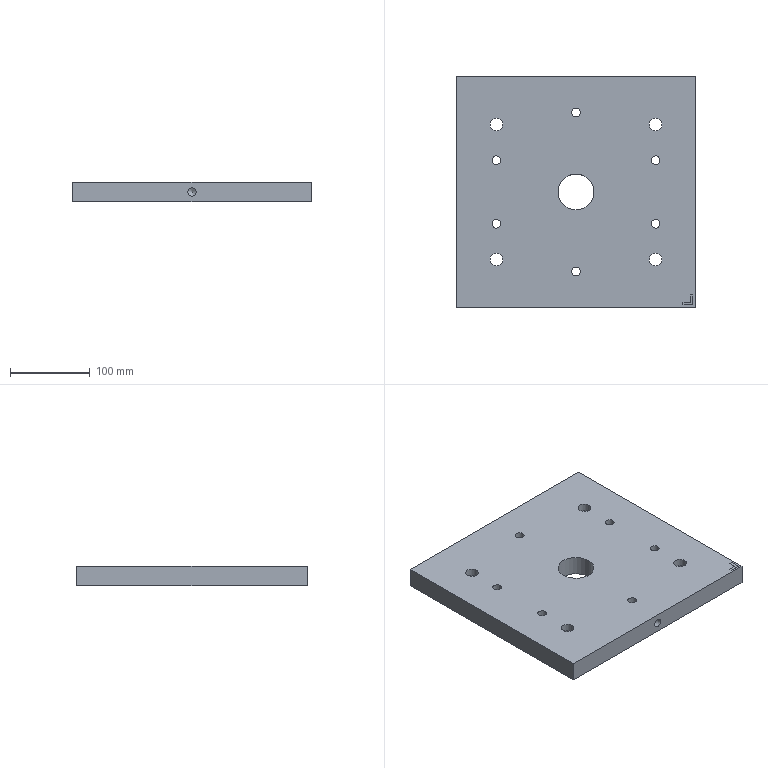Part | STEP file | BD_id262_x_t | 1 solid | 48 faces | box 300 x 290 x 25 mm | volume 2072800 mm3 | plane 23 | cylinder 23 | cone 2 | commonest cylinder face diameters 11 x6 18 x6 16 x4 23 x4 10.5 x2 45 x1
STEP:
#1=CARTESIAN_POINT('',(9.,100.,-190.5));
#2=VERTEX_POINT('',#1);
#3=CARTESIAN_POINT('',(0.,100.,-190.5));
#4=DIRECTION('',(0.,0.,1.));
#5=DIRECTION('',(1.,0.,0.));
#6=AXIS2_PLACEMENT_3D('',#3,#4,#5);
#7=CIRCLE('',#6,9.);
#8=EDGE_CURVE('',#2,#2,#7,.T.);
#9=ORIENTED_EDGE('',*,*,#8,.T.);
#10=EDGE_LOOP('',(#9));
#11=FACE_BOUND('',#10,.T.);
#12=CARTESIAN_POINT('',(-109.,-40.,-190.5));
#13=VERTEX_POINT('',#12);
#14=CARTESIAN_POINT('',(-100.,-40.,-190.5));
#15=DIRECTION('',(0.,0.,1.));
#16=DIRECTION('',(-1.,0.,0.));
#17=AXIS2_PLACEMENT_3D('',#14,#15,#16);
#18=CIRCLE('',#17,9.);
#19=EDGE_CURVE('',#13,#13,#18,.T.);
#20=ORIENTED_EDGE('',*,*,#19,.T.);
#21=EDGE_LOOP('',(#20));
#22=FACE_BOUND('',#21,.T.);
#23=CARTESIAN_POINT('',(109.,-40.,-190.5));
#24=VERTEX_POINT('',#23);
#25=CARTESIAN_POINT('',(100.,-40.,-190.5));
#26=DIRECTION('',(0.,0.,1.));
#27=DIRECTION('',(1.,0.,0.));
#28=AXIS2_PLACEMENT_3D('',#25,#26,#27);
#29=CIRCLE('',#28,9.);
#30=EDGE_CURVE('',#24,#24,#29,.T.);
#31=ORIENTED_EDGE('',*,*,#30,.T.);
#32=EDGE_LOOP('',(#31));
#33=FACE_BOUND('',#32,.T.);
#34=CARTESIAN_POINT('',(-111.5,-85.,-190.5));
#35=VERTEX_POINT('',#34);
#36=CARTESIAN_POINT('',(-100.,-85.,-190.5));
#37=DIRECTION('',(0.,0.,1.));
#38=DIRECTION('',(-1.,0.,0.));
#39=AXIS2_PLACEMENT_3D('',#36,#37,#38);
#40=CIRCLE('',#39,11.5);
#41=EDGE_CURVE('',#35,#35,#40,.T.);
#42=ORIENTED_EDGE('',*,*,#41,.T.);
#43=EDGE_LOOP('',(#42));
#44=FACE_BOUND('',#43,.T.);
#45=CARTESIAN_POINT('',(111.5,85.,-190.5));
#46=VERTEX_POINT('',#45);
#47=CARTESIAN_POINT('',(100.,85.,-190.5));
#48=DIRECTION('',(0.,0.,1.));
#49=DIRECTION('',(1.,0.,0.));
#50=AXIS2_PLACEMENT_3D('',#47,#48,#49);
#51=CIRCLE('',#50,11.5);
#52=EDGE_CURVE('',#46,#46,#51,.T.);
#53=ORIENTED_EDGE('',*,*,#52,.T.);
#54=EDGE_LOOP('',(#53));
#55=FACE_BOUND('',#54,.T.);
#56=CARTESIAN_POINT('',(150.,-145.,-190.5));
#57=VERTEX_POINT('',#56);
#58=CARTESIAN_POINT('',(150.,145.,-190.5));
#59=VERTEX_POINT('',#58);
#60=CARTESIAN_POINT('',(150.,0.,-190.5));
#61=DIRECTION('',(0.,1.,0.));
#62=VECTOR('',#61,1.);
#63=LINE('',#60,#62);
#64=EDGE_CURVE('',#57,#59,#63,.T.);
#65=ORIENTED_EDGE('',*,*,#64,.F.);
#66=CARTESIAN_POINT('',(-150.,-145.,-190.5));
#67=VERTEX_POINT('',#66);
#68=CARTESIAN_POINT('',(0.,-145.,-190.5));
#69=DIRECTION('',(1.,0.,0.));
#70=VECTOR('',#69,1.);
#71=LINE('',#68,#70);
#72=EDGE_CURVE('',#67,#57,#71,.T.);
#73=ORIENTED_EDGE('',*,*,#72,.F.);
#74=CARTESIAN_POINT('',(-150.,145.,-190.5));
#75=VERTEX_POINT('',#74);
#76=CARTESIAN_POINT('',(-150.,0.,-190.5));
#77=DIRECTION('',(0.,-1.,0.));
#78=VECTOR('',#77,1.);
#79=LINE('',#76,#78);
#80=EDGE_CURVE('',#75,#67,#79,.T.);
#81=ORIENTED_EDGE('',*,*,#80,.F.);
#82=CARTESIAN_POINT('',(0.,145.,-190.5));
#83=DIRECTION('',(-1.,0.,0.));
#84=VECTOR('',#83,1.);
#85=LINE('',#82,#84);
#86=EDGE_CURVE('',#59,#75,#85,.T.);
#87=ORIENTED_EDGE('',*,*,#86,.F.);
#88=EDGE_LOOP('',(#65,#73,#81,#87));
#89=FACE_BOUND('',#88,.T.);
#90=CARTESIAN_POINT('',(111.5,-85.,-190.5));
#91=VERTEX_POINT('',#90);
#92=CARTESIAN_POINT('',(100.,-85.,-190.5));
#93=DIRECTION('',(0.,0.,1.));
#94=DIRECTION('',(1.,0.,0.));
#95=AXIS2_PLACEMENT_3D('',#92,#93,#94);
#96=CIRCLE('',#95,11.5);
#97=EDGE_CURVE('',#91,#91,#96,.T.);
#98=ORIENTED_EDGE('',*,*,#97,.T.);
#99=EDGE_LOOP('',(#98));
#100=FACE_BOUND('',#99,.T.);
#101=CARTESIAN_POINT('',(-88.5,85.,-190.5));
#102=VERTEX_POINT('',#101);
#103=CARTESIAN_POINT('',(-100.,85.,-190.5));
#104=DIRECTION('',(0.,0.,1.));
#105=DIRECTION('',(1.,0.,0.));
#106=AXIS2_PLACEMENT_3D('',#103,#104,#105);
#107=CIRCLE('',#106,11.5);
#108=EDGE_CURVE('',#102,#102,#107,.T.);
#109=ORIENTED_EDGE('',*,*,#108,.T.);
#110=EDGE_LOOP('',(#109));
#111=FACE_BOUND('',#110,.T.);
#112=CARTESIAN_POINT('',(109.,40.,-190.5));
#113=VERTEX_POINT('',#112);
#114=CARTESIAN_POINT('',(100.,40.,-190.5));
#115=DIRECTION('',(0.,0.,1.));
#116=DIRECTION('',(1.,0.,0.));
#117=AXIS2_PLACEMENT_3D('',#114,#115,#116);
#118=CIRCLE('',#117,9.);
#119=EDGE_CURVE('',#113,#113,#118,.T.);
#120=ORIENTED_EDGE('',*,*,#119,.T.);
#121=EDGE_LOOP('',(#120));
#122=FACE_BOUND('',#121,.T.);
#123=CARTESIAN_POINT('',(-91.,40.,-190.5));
#124=VERTEX_POINT('',#123);
#125=CARTESIAN_POINT('',(-100.,40.,-190.5));
#126=DIRECTION('',(0.,0.,1.));
#127=DIRECTION('',(1.,0.,0.));
#128=AXIS2_PLACEMENT_3D('',#125,#126,#127);
#129=CIRCLE('',#128,9.);
#130=EDGE_CURVE('',#124,#124,#129,.T.);
#131=ORIENTED_EDGE('',*,*,#130,.T.);
#132=EDGE_LOOP('',(#131));
#133=FACE_BOUND('',#132,.T.);
#134=CARTESIAN_POINT('',(-22.5,0.,-190.5));
#135=VERTEX_POINT('',#134);
#136=CARTESIAN_POINT('',(0.,0.,-190.5));
#137=DIRECTION('',(0.,0.,1.));
#138=DIRECTION('',(-1.,0.,0.));
#139=AXIS2_PLACEMENT_3D('',#136,#137,#138);
#140=CIRCLE('',#139,22.5);
#141=EDGE_CURVE('',#135,#135,#140,.T.);
#142=ORIENTED_EDGE('',*,*,#141,.T.);
#143=EDGE_LOOP('',(#142));
#144=FACE_BOUND('',#143,.T.);
#145=CARTESIAN_POINT('',(9.,-100.,-190.5));
#146=VERTEX_POINT('',#145);
#147=CARTESIAN_POINT('',(0.,-100.,-190.5));
#148=DIRECTION('',(0.,0.,1.));
#149=DIRECTION('',(1.,0.,0.));
#150=AXIS2_PLACEMENT_3D('',#147,#148,#149);
#151=CIRCLE('',#150,9.);
#152=EDGE_CURVE('',#146,#146,#151,.T.);
#153=ORIENTED_EDGE('',*,*,#152,.T.);
#154=EDGE_LOOP('',(#153));
#155=FACE_BOUND('',#154,.T.);
#156=CARTESIAN_POINT('',(0.,0.,-190.5));
#157=DIRECTION('',(0.,0.,-1.));
#158=DIRECTION('',(-1.,0.,0.));
#159=AXIS2_PLACEMENT_3D('',#156,#157,#158);
#160=PLANE('',#159);
#161=ADVANCED_FACE('',(#11,#22,#33,#44,#55,#89,#100,#111,#122,#133,#144,#155),#160,.T.);
#162=CARTESIAN_POINT('',(-5.5,100.,-165.5));
#163=VERTEX_POINT('',#162);
#164=CARTESIAN_POINT('',(0.,100.,-165.5));
#165=DIRECTION('',(0.,0.,-1.));
#166=DIRECTION('',(-1.,0.,0.));
#167=AXIS2_PLACEMENT_3D('',#164,#165,#166);
#168=CIRCLE('',#167,5.5);
#169=EDGE_CURVE('',#163,#163,#168,.T.);
#170=ORIENTED_EDGE('',*,*,#169,.T.);
#171=EDGE_LOOP('',(#170));
#172=FACE_BOUND('',#171,.T.);
#173=CARTESIAN_POINT('',(-94.5,-40.,-165.5));
#174=VERTEX_POINT('',#173);
#175=CARTESIAN_POINT('',(-100.,-40.,-165.5));
#176=DIRECTION('',(0.,0.,-1.));
#177=DIRECTION('',(1.,0.,0.));
#178=AXIS2_PLACEMENT_3D('',#175,#176,#177);
#179=CIRCLE('',#178,5.5);
#180=EDGE_CURVE('',#174,#174,#179,.T.);
#181=ORIENTED_EDGE('',*,*,#180,.T.);
#182=EDGE_LOOP('',(#181));
#183=FACE_BOUND('',#182,.T.);
#184=CARTESIAN_POINT('',(94.5,-40.,-165.5));
#185=VERTEX_POINT('',#184);
#186=CARTESIAN_POINT('',(100.,-40.,-165.5));
#187=DIRECTION('',(0.,0.,-1.));
#188=DIRECTION('',(-1.,0.,0.));
#189=AXIS2_PLACEMENT_3D('',#186,#187,#188);
#190=CIRCLE('',#189,5.5);
#191=EDGE_CURVE('',#185,#185,#190,.T.);
#192=ORIENTED_EDGE('',*,*,#191,.T.);
#193=EDGE_LOOP('',(#192));
#194=FACE_BOUND('',#193,.T.);
#195=CARTESIAN_POINT('',(-92.,-85.,-165.5));
#196=VERTEX_POINT('',#195);
#197=CARTESIAN_POINT('',(-100.,-85.,-165.5));
#198=DIRECTION('',(0.,0.,-1.));
#199=DIRECTION('',(1.,0.,0.));
#200=AXIS2_PLACEMENT_3D('',#197,#198,#199);
#201=CIRCLE('',#200,8.);
#202=EDGE_CURVE('',#196,#196,#201,.T.);
#203=ORIENTED_EDGE('',*,*,#202,.T.);
#204=EDGE_LOOP('',(#203));
#205=FACE_BOUND('',#204,.T.);
#206=CARTESIAN_POINT('',(92.,85.,-165.5));
#207=VERTEX_POINT('',#206);
#208=CARTESIAN_POINT('',(100.,85.,-165.5));
#209=DIRECTION('',(0.,0.,-1.));
#210=DIRECTION('',(-1.,0.,0.));
#211=AXIS2_PLACEMENT_3D('',#208,#209,#210);
#212=CIRCLE('',#211,8.);
#213=EDGE_CURVE('',#207,#207,#212,.T.);
#214=ORIENTED_EDGE('',*,*,#213,.T.);
#215=EDGE_LOOP('',(#214));
#216=FACE_BOUND('',#215,.T.);
#217=CARTESIAN_POINT('',(143.75,-129.375,-165.5));
#218=VERTEX_POINT('',#217);
#219=CARTESIAN_POINT('',(143.75,-138.75,-165.5));
#220=VERTEX_POINT('',#219);
#221=CARTESIAN_POINT('',(143.75,-134.062,-165.5));
#222=DIRECTION('',(0.,-1.,0.));
#223=VECTOR('',#222,1.);
#224=LINE('',#221,#223);
#225=EDGE_CURVE('',#218,#220,#224,.T.);
#226=ORIENTED_EDGE('',*,*,#225,.F.);
#227=CARTESIAN_POINT('',(146.875,-129.375,-165.5));
#228=VERTEX_POINT('',#227);
#229=CARTESIAN_POINT('',(140.625,-129.375,-165.5));
#230=DIRECTION('',(1.,0.,0.));
#231=VECTOR('',#230,1.);
#232=LINE('',#229,#231);
#233=EDGE_CURVE('',#218,#228,#232,.T.);
#234=ORIENTED_EDGE('',*,*,#233,.T.);
#235=CARTESIAN_POINT('',(146.875,-141.875,-165.5));
#236=VERTEX_POINT('',#235);
#237=CARTESIAN_POINT('',(146.875,-135.625,-165.5));
#238=DIRECTION('',(0.,-1.,0.));
#239=VECTOR('',#238,1.);
#240=LINE('',#237,#239);
#241=EDGE_CURVE('',#228,#236,#240,.T.);
#242=ORIENTED_EDGE('',*,*,#241,.T.);
#243=CARTESIAN_POINT('',(134.375,-141.875,-165.5));
#244=VERTEX_POINT('',#243);
#245=CARTESIAN_POINT('',(140.625,-141.875,-165.5));
#246=DIRECTION('',(-1.,0.,0.));
#247=VECTOR('',#246,1.);
#248=LINE('',#245,#247);
#249=EDGE_CURVE('',#236,#244,#248,.T.);
#250=ORIENTED_EDGE('',*,*,#249,.T.);
#251=CARTESIAN_POINT('',(134.375,-138.75,-165.5));
#252=VERTEX_POINT('',#251);
#253=CARTESIAN_POINT('',(134.375,-135.625,-165.5));
#254=DIRECTION('',(0.,1.,0.));
#255=VECTOR('',#254,1.);
#256=LINE('',#253,#255);
#257=EDGE_CURVE('',#244,#252,#256,.T.);
#258=ORIENTED_EDGE('',*,*,#257,.T.);
#259=CARTESIAN_POINT('',(139.062,-138.75,-165.5));
#260=DIRECTION('',(-1.,0.,0.));
#261=VECTOR('',#260,1.);
#262=LINE('',#259,#261);
#263=EDGE_CURVE('',#220,#252,#262,.T.);
#264=ORIENTED_EDGE('',*,*,#263,.F.);
#265=EDGE_LOOP('',(#226,#234,#242,#250,#258,#264));
#266=FACE_BOUND('',#265,.T.);
#267=CARTESIAN_POINT('',(150.,-145.,-165.5));
#268=VERTEX_POINT('',#267);
#269=CARTESIAN_POINT('',(-150.,-145.,-165.5));
#270=VERTEX_POINT('',#269);
#271=CARTESIAN_POINT('',(0.,-145.,-165.5));
#272=DIRECTION('',(-1.,0.,0.));
#273=VECTOR('',#272,1.);
#274=LINE('',#271,#273);
#275=EDGE_CURVE('',#268,#270,#274,.T.);
#276=ORIENTED_EDGE('',*,*,#275,.F.);
#277=CARTESIAN_POINT('',(150.,145.,-165.5));
#278=VERTEX_POINT('',#277);
#279=CARTESIAN_POINT('',(150.,0.,-165.5));
#280=DIRECTION('',(0.,-1.,0.));
#281=VECTOR('',#280,1.);
#282=LINE('',#279,#281);
#283=EDGE_CURVE('',#278,#268,#282,.T.);
#284=ORIENTED_EDGE('',*,*,#283,.F.);
#285=CARTESIAN_POINT('',(-150.,145.,-165.5));
#286=VERTEX_POINT('',#285);
#287=CARTESIAN_POINT('',(0.,145.,-165.5));
#288=DIRECTION('',(1.,0.,0.));
#289=VECTOR('',#288,1.);
#290=LINE('',#287,#289);
#291=EDGE_CURVE('',#286,#278,#290,.T.);
#292=ORIENTED_EDGE('',*,*,#291,.F.);
#293=CARTESIAN_POINT('',(-150.,0.,-165.5));
#294=DIRECTION('',(0.,1.,0.));
#295=VECTOR('',#294,1.);
#296=LINE('',#293,#295);
#297=EDGE_CURVE('',#270,#286,#296,.T.);
#298=ORIENTED_EDGE('',*,*,#297,.F.);
#299=EDGE_LOOP('',(#276,#284,#292,#298));
#300=FACE_BOUND('',#299,.T.);
#301=CARTESIAN_POINT('',(92.,-85.,-165.5));
#302=VERTEX_POINT('',#301);
#303=CARTESIAN_POINT('',(100.,-85.,-165.5));
#304=DIRECTION('',(0.,0.,-1.));
#305=DIRECTION('',(-1.,0.,0.));
#306=AXIS2_PLACEMENT_3D('',#303,#304,#305);
#307=CIRCLE('',#306,8.);
#308=EDGE_CURVE('',#302,#302,#307,.T.);
#309=ORIENTED_EDGE('',*,*,#308,.T.);
#310=EDGE_LOOP('',(#309));
#311=FACE_BOUND('',#310,.T.);
#312=CARTESIAN_POINT('',(-108.,85.,-165.5));
#313=VERTEX_POINT('',#312);
#314=CARTESIAN_POINT('',(-100.,85.,-165.5));
#315=DIRECTION('',(0.,0.,-1.));
#316=DIRECTION('',(-1.,0.,0.));
#317=AXIS2_PLACEMENT_3D('',#314,#315,#316);
#318=CIRCLE('',#317,8.);
#319=EDGE_CURVE('',#313,#313,#318,.T.);
#320=ORIENTED_EDGE('',*,*,#319,.T.);
#321=EDGE_LOOP('',(#320));
#322=FACE_BOUND('',#321,.T.);
#323=CARTESIAN_POINT('',(94.5,40.,-165.5));
#324=VERTEX_POINT('',#323);
#325=CARTESIAN_POINT('',(100.,40.,-165.5));
#326=DIRECTION('',(0.,0.,-1.));
#327=DIRECTION('',(-1.,0.,0.));
#328=AXIS2_PLACEMENT_3D('',#325,#326,#327);
#329=CIRCLE('',#328,5.5);
#330=EDGE_CURVE('',#324,#324,#329,.T.);
#331=ORIENTED_EDGE('',*,*,#330,.T.);
#332=EDGE_LOOP('',(#331));
#333=FACE_BOUND('',#332,.T.);
#334=CARTESIAN_POINT('',(-105.5,40.,-165.5));
#335=VERTEX_POINT('',#334);
#336=CARTESIAN_POINT('',(-100.,40.,-165.5));
#337=DIRECTION('',(0.,0.,-1.));
#338=DIRECTION('',(-1.,0.,0.));
#339=AXIS2_PLACEMENT_3D('',#336,#337,#338);
#340=CIRCLE('',#339,5.5);
#341=EDGE_CURVE('',#335,#335,#340,.T.);
#342=ORIENTED_EDGE('',*,*,#341,.T.);
#343=EDGE_LOOP('',(#342));
#344=FACE_BOUND('',#343,.T.);
#345=CARTESIAN_POINT('',(22.5,0.,-165.5));
#346=VERTEX_POINT('',#345);
#347=CARTESIAN_POINT('',(0.,0.,-165.5));
#348=DIRECTION('',(0.,0.,-1.));
#349=DIRECTION('',(1.,0.,0.));
#350=AXIS2_PLACEMENT_3D('',#347,#348,#349);
#351=CIRCLE('',#350,22.5);
#352=EDGE_CURVE('',#346,#346,#351,.T.);
#353=ORIENTED_EDGE('',*,*,#352,.T.);
#354=EDGE_LOOP('',(#353));
#355=FACE_BOUND('',#354,.T.);
#356=CARTESIAN_POINT('',(-5.5,-100.,-165.5));
#357=VERTEX_POINT('',#356);
#358=CARTESIAN_POINT('',(0.,-100.,-165.5));
#359=DIRECTION('',(0.,0.,-1.));
#360=DIRECTION('',(-1.,0.,0.));
#361=AXIS2_PLACEMENT_3D('',#358,#359,#360);
#362=CIRCLE('',#361,5.5);
#363=EDGE_CURVE('',#357,#357,#362,.T.);
#364=ORIENTED_EDGE('',*,*,#363,.T.);
#365=EDGE_LOOP('',(#364));
#366=FACE_BOUND('',#365,.T.);
#367=CARTESIAN_POINT('',(0.,0.,-165.5));
#368=DIRECTION('',(0.,0.,1.));
#369=DIRECTION('',(1.,0.,0.));
#370=AXIS2_PLACEMENT_3D('',#367,#368,#369);
#371=PLANE('',#370);
#372=ADVANCED_FACE('',(#172,#183,#194,#205,#216,#266,#300,#311,#322,#333,#344,#355,#366),#371,.T.);
#373=CARTESIAN_POINT('',(0.,-145.,-172.75));
#374=VERTEX_POINT('',#373);
#375=CARTESIAN_POINT('',(0.,-145.,-178.));
#376=DIRECTION('',(0.,1.,0.));
#377=DIRECTION('',(0.,0.,1.));
#378=AXIS2_PLACEMENT_3D('',#375,#376,#377);
#379=CIRCLE('',#378,5.25);
#380=EDGE_CURVE('',#374,#374,#379,.T.);
#381=ORIENTED_EDGE('',*,*,#380,.T.);
#382=EDGE_LOOP('',(#381));
#383=FACE_BOUND('',#382,.T.);
#384=CARTESIAN_POINT('',(150.,-145.,-190.5));
#385=DIRECTION('',(0.,0.,1.));
#386=VECTOR('',#385,1.);
#387=LINE('',#384,#386);
#388=EDGE_CURVE('',#57,#268,#387,.T.);
#389=ORIENTED_EDGE('',*,*,#388,.T.);
#390=ORIENTED_EDGE('',*,*,#275,.T.);
#391=CARTESIAN_POINT('',(-150.,-145.,-190.5));
#392=DIRECTION('',(0.,0.,1.));
#393=VECTOR('',#392,1.);
#394=LINE('',#391,#393);
#395=EDGE_CURVE('',#67,#270,#394,.T.);
#396=ORIENTED_EDGE('',*,*,#395,.F.);
#397=ORIENTED_EDGE('',*,*,#72,.T.);
#398=EDGE_LOOP('',(#389,#390,#396,#397));
#399=FACE_BOUND('',#398,.T.);
#400=CARTESIAN_POINT('',(0.,-145.,-190.5));
#401=DIRECTION('',(0.,-1.,0.));
#402=DIRECTION('',(0.,0.,-1.));
#403=AXIS2_PLACEMENT_3D('',#400,#401,#402);
#404=PLANE('',#403);
#405=ADVANCED_FACE('',(#383,#399),#404,.T.);
#406=ORIENTED_EDGE('',*,*,#395,.T.);
#407=ORIENTED_EDGE('',*,*,#297,.T.);
#408=CARTESIAN_POINT('',(-150.,145.,-190.5));
#409=DIRECTION('',(0.,0.,1.));
#410=VECTOR('',#409,1.);
#411=LINE('',#408,#410);
#412=EDGE_CURVE('',#75,#286,#411,.T.);
#413=ORIENTED_EDGE('',*,*,#412,.F.);
#414=ORIENTED_EDGE('',*,*,#80,.T.);
#415=EDGE_LOOP('',(#406,#407,#413,#414));
#416=FACE_OUTER_BOUND('',#415,.T.);
#417=CARTESIAN_POINT('',(-150.,0.,-190.5));
#418=DIRECTION('',(-1.,0.,0.));
#419=DIRECTION('',(0.,0.,1.));
#420=AXIS2_PLACEMENT_3D('',#417,#418,#419);
#421=PLANE('',#420);
#422=ADVANCED_FACE('',(#416),#421,.T.);
#423=CARTESIAN_POINT('',(0.,145.,-183.25));
#424=VERTEX_POINT('',#423);
#425=CARTESIAN_POINT('',(0.,145.,-178.));
#426=DIRECTION('',(0.,-1.,0.));
#427=DIRECTION('',(0.,0.,-1.));
#428=AXIS2_PLACEMENT_3D('',#425,#426,#427);
#429=CIRCLE('',#428,5.25);
#430=EDGE_CURVE('',#424,#424,#429,.T.);
#431=ORIENTED_EDGE('',*,*,#430,.T.);
#432=EDGE_LOOP('',(#431));
#433=FACE_BOUND('',#432,.T.);
#434=ORIENTED_EDGE('',*,*,#412,.T.);
#435=ORIENTED_EDGE('',*,*,#291,.T.);
#436=CARTESIAN_POINT('',(150.,145.,-190.5));
#437=DIRECTION('',(0.,0.,1.));
#438=VECTOR('',#437,1.);
#439=LINE('',#436,#438);
#440=EDGE_CURVE('',#59,#278,#439,.T.);
#441=ORIENTED_EDGE('',*,*,#440,.F.);
#442=ORIENTED_EDGE('',*,*,#86,.T.);
#443=EDGE_LOOP('',(#434,#435,#441,#442));
#444=FACE_BOUND('',#443,.T.);
#445=CARTESIAN_POINT('',(0.,145.,-190.5));
#446=DIRECTION('',(0.,1.,0.));
#447=DIRECTION('',(0.,0.,1.));
#448=AXIS2_PLACEMENT_3D('',#445,#446,#447);
#449=PLANE('',#448);
#450=ADVANCED_FACE('',(#433,#444),#449,.T.);
#451=ORIENTED_EDGE('',*,*,#64,.T.);
#452=ORIENTED_EDGE('',*,*,#440,.T.);
#453=ORIENTED_EDGE('',*,*,#283,.T.);
#454=ORIENTED_EDGE('',*,*,#388,.F.);
#455=EDGE_LOOP('',(#451,#452,#453,#454));
#456=FACE_OUTER_BOUND('',#455,.T.);
#457=CARTESIAN_POINT('',(150.,0.,-190.5));
#458=DIRECTION('',(1.,0.,0.));
#459=DIRECTION('',(0.,0.,-1.));
#460=AXIS2_PLACEMENT_3D('',#457,#458,#459);
#461=PLANE('',#460);
#462=ADVANCED_FACE('',(#456),#461,.T.);
#463=CARTESIAN_POINT('',(146.875,-129.375,-165.6));
#464=VERTEX_POINT('',#463);
#465=CARTESIAN_POINT('',(143.75,-129.375,-165.6));
#466=VERTEX_POINT('',#465);
#467=CARTESIAN_POINT('',(140.625,-129.375,-165.6));
#468=DIRECTION('',(-1.,0.,0.));
#469=VECTOR('',#468,1.);
#470=LINE('',#467,#469);
#471=EDGE_CURVE('',#464,#466,#470,.T.);
#472=ORIENTED_EDGE('',*,*,#471,.F.);
#473=CARTESIAN_POINT('',(146.875,-129.375,-165.6));
#474=DIRECTION('',(0.,0.,1.));
#475=VECTOR('',#474,1.);
#476=LINE('',#473,#475);
#477=EDGE_CURVE('',#464,#228,#476,.T.);
#478=ORIENTED_EDGE('',*,*,#477,.T.);
#479=ORIENTED_EDGE('',*,*,#233,.F.);
#480=CARTESIAN_POINT('',(143.75,-129.375,-165.6));
#481=DIRECTION('',(0.,0.,1.));
#482=VECTOR('',#481,1.);
#483=LINE('',#480,#482);
#484=EDGE_CURVE('',#466,#218,#483,.T.);
#485=ORIENTED_EDGE('',*,*,#484,.F.);
#486=EDGE_LOOP('',(#472,#478,#479,#485));
#487=FACE_OUTER_BOUND('',#486,.T.);
#488=CARTESIAN_POINT('',(140.625,-129.375,-165.6));
#489=DIRECTION('',(0.,1.,0.));
#490=DIRECTION('',(0.,0.,1.));
#491=AXIS2_PLACEMENT_3D('',#488,#489,#490);
#492=PLANE('',#491);
#493=ADVANCED_FACE('',(#487),#492,.F.);
#494=CARTESIAN_POINT('',(134.375,-138.75,-165.6));
#495=VERTEX_POINT('',#494);
#496=CARTESIAN_POINT('',(143.75,-138.75,-165.6));
#497=VERTEX_POINT('',#496);
#498=CARTESIAN_POINT('',(139.062,-138.75,-165.6));
#499=DIRECTION('',(1.,0.,0.));
#500=VECTOR('',#499,1.);
#501=LINE('',#498,#500);
#502=EDGE_CURVE('',#495,#497,#501,.T.);
#503=ORIENTED_EDGE('',*,*,#502,.F.);
#504=CARTESIAN_POINT('',(134.375,-141.875,-165.6));
#505=VERTEX_POINT('',#504);
#506=CARTESIAN_POINT('',(134.375,-135.625,-165.6));
#507=DIRECTION('',(0.,-1.,0.));
#508=VECTOR('',#507,1.);
#509=LINE('',#506,#508);
#510=EDGE_CURVE('',#495,#505,#509,.T.);
#511=ORIENTED_EDGE('',*,*,#510,.T.);
#512=CARTESIAN_POINT('',(146.875,-141.875,-165.6));
#513=VERTEX_POINT('',#512);
#514=CARTESIAN_POINT('',(140.625,-141.875,-165.6));
#515=DIRECTION('',(1.,0.,0.));
#516=VECTOR('',#515,1.);
#517=LINE('',#514,#516);
#518=EDGE_CURVE('',#505,#513,#517,.T.);
#519=ORIENTED_EDGE('',*,*,#518,.T.);
#520=CARTESIAN_POINT('',(146.875,-135.625,-165.6));
#521=DIRECTION('',(0.,1.,0.));
#522=VECTOR('',#521,1.);
#523=LINE('',#520,#522);
#524=EDGE_CURVE('',#513,#464,#523,.T.);
#525=ORIENTED_EDGE('',*,*,#524,.T.);
#526=ORIENTED_EDGE('',*,*,#471,.T.);
#527=CARTESIAN_POINT('',(143.75,-134.062,-165.6));
#528=DIRECTION('',(0.,1.,0.));
#529=VECTOR('',#528,1.);
#530=LINE('',#527,#529);
#531=EDGE_CURVE('',#497,#466,#530,.T.);
#532=ORIENTED_EDGE('',*,*,#531,.F.);
#533=EDGE_LOOP('',(#503,#511,#519,#525,#526,#532));
#534=FACE_OUTER_BOUND('',#533,.T.);
#535=CARTESIAN_POINT('',(140.625,-135.625,-165.6));
#536=DIRECTION('',(0.,0.,-1.));
#537=DIRECTION('',(-1.,0.,0.));
#538=AXIS2_PLACEMENT_3D('',#535,#536,#537);
#539=PLANE('',#538);
#540=ADVANCED_FACE('',(#534),#539,.F.);
#541=CARTESIAN_POINT('',(146.875,-141.875,-165.6));
#542=DIRECTION('',(0.,0.,1.));
#543=VECTOR('',#542,1.);
#544=LINE('',#541,#543);
#545=EDGE_CURVE('',#513,#236,#544,.T.);
#546=ORIENTED_EDGE('',*,*,#545,.F.);
#547=ORIENTED_EDGE('',*,*,#518,.F.);
#548=CARTESIAN_POINT('',(134.375,-141.875,-165.6));
#549=DIRECTION('',(0.,0.,1.));
#550=VECTOR('',#549,1.);
#551=LINE('',#548,#550);
#552=EDGE_CURVE('',#505,#244,#551,.T.);
#553=ORIENTED_EDGE('',*,*,#552,.T.);
#554=ORIENTED_EDGE('',*,*,#249,.F.);
#555=EDGE_LOOP('',(#546,#547,#553,#554));
#556=FACE_OUTER_BOUND('',#555,.T.);
#557=CARTESIAN_POINT('',(140.625,-141.875,-165.6));
#558=DIRECTION('',(0.,-1.,0.));
#559=DIRECTION('',(0.,0.,-1.));
#560=AXIS2_PLACEMENT_3D('',#557,#558,#559);
#561=PLANE('',#560);
#562=ADVANCED_FACE('',(#556),#561,.F.);
#563=CARTESIAN_POINT('',(134.375,-138.75,-165.6));
#564=DIRECTION('',(0.,0.,1.));
#565=VECTOR('',#564,1.);
#566=LINE('',#563,#565);
#567=EDGE_CURVE('',#495,#252,#566,.T.);
#568=ORIENTED_EDGE('',*,*,#567,.T.);
#569=ORIENTED_EDGE('',*,*,#257,.F.);
#570=ORIENTED_EDGE('',*,*,#552,.F.);
#571=ORIENTED_EDGE('',*,*,#510,.F.);
#572=EDGE_LOOP('',(#568,#569,#570,#571));
#573=FACE_OUTER_BOUND('',#572,.T.);
#574=CARTESIAN_POINT('',(134.375,-135.625,-165.6));
#575=DIRECTION('',(-1.,0.,0.));
#576=DIRECTION('',(0.,0.,1.));
#577=AXIS2_PLACEMENT_3D('',#574,#575,#576);
#578=PLANE('',#577);
#579=ADVANCED_FACE('',(#573),#578,.F.);
#580=ORIENTED_EDGE('',*,*,#524,.F.);
#581=ORIENTED_EDGE('',*,*,#545,.T.);
#582=ORIENTED_EDGE('',*,*,#241,.F.);
#583=ORIENTED_EDGE('',*,*,#477,.F.);
#584=EDGE_LOOP('',(#580,#581,#582,#583));
#585=FACE_OUTER_BOUND('',#584,.T.);
#586=CARTESIAN_POINT('',(146.875,-135.625,-165.6));
#587=DIRECTION('',(1.,0.,0.));
#588=DIRECTION('',(0.,0.,-1.));
#589=AXIS2_PLACEMENT_3D('',#586,#587,#588);
#590=PLANE('',#589);
#591=ADVANCED_FACE('',(#585),#590,.F.);
#592=CARTESIAN_POINT('',(143.75,-138.75,-165.6));
#593=DIRECTION('',(0.,0.,1.));
#594=VECTOR('',#593,1.);
#595=LINE('',#592,#594);
#596=EDGE_CURVE('',#497,#220,#595,.T.);
#597=ORIENTED_EDGE('',*,*,#596,.T.);
#598=ORIENTED_EDGE('',*,*,#263,.T.);
#599=ORIENTED_EDGE('',*,*,#567,.F.);
#600=ORIENTED_EDGE('',*,*,#502,.T.);
#601=EDGE_LOOP('',(#597,#598,#599,#600));
#602=FACE_OUTER_BOUND('',#601,.T.);
#603=CARTESIAN_POINT('',(139.062,-138.75,-165.6));
#604=DIRECTION('',(0.,-1.,0.));
#605=DIRECTION('',(0.,0.,-1.));
#606=AXIS2_PLACEMENT_3D('',#603,#604,#605);
#607=PLANE('',#606);
#608=ADVANCED_FACE('',(#602),#607,.T.);
#609=ORIENTED_EDGE('',*,*,#531,.T.);
#610=ORIENTED_EDGE('',*,*,#484,.T.);
#611=ORIENTED_EDGE('',*,*,#225,.T.);
#612=ORIENTED_EDGE('',*,*,#596,.F.);
#613=EDGE_LOOP('',(#609,#610,#611,#612));
#614=FACE_OUTER_BOUND('',#613,.T.);
#615=CARTESIAN_POINT('',(143.75,-134.062,-165.6));
#616=DIRECTION('',(1.,0.,0.));
#617=DIRECTION('',(0.,0.,-1.));
#618=AXIS2_PLACEMENT_3D('',#615,#616,#617);
#619=PLANE('',#618);
#620=ADVANCED_FACE('',(#614),#619,.T.);
#621=CARTESIAN_POINT('',(108.,85.,-175.3));
#622=VERTEX_POINT('',#621);
#623=CARTESIAN_POINT('',(100.,85.,-175.3));
#624=DIRECTION('',(0.,0.,-1.));
#625=DIRECTION('',(1.,0.,0.));
#626=AXIS2_PLACEMENT_3D('',#623,#624,#625);
#627=CIRCLE('',#626,8.);
#628=EDGE_CURVE('',#622,#622,#627,.T.);
#629=ORIENTED_EDGE('',*,*,#628,.T.);
#630=EDGE_LOOP('',(#629));
#631=FACE_BOUND('',#630,.T.);
#632=ORIENTED_EDGE('',*,*,#213,.F.);
#633=EDGE_LOOP('',(#632));
#634=FACE_BOUND('',#633,.T.);
#635=CARTESIAN_POINT('',(100.,85.,-190.5));
#636=DIRECTION('',(0.,0.,1.));
#637=DIRECTION('',(1.,0.,0.));
#638=AXIS2_PLACEMENT_3D('',#635,#636,#637);
#639=CYLINDRICAL_SURFACE('',#638,8.);
#640=ADVANCED_FACE('',(#631,#634),#639,.F.);
#641=ORIENTED_EDGE('',*,*,#628,.F.);
#642=EDGE_LOOP('',(#641));
#643=FACE_BOUND('',#642,.T.);
#644=CARTESIAN_POINT('',(88.5,85.,-175.3));
#645=VERTEX_POINT('',#644);
#646=CARTESIAN_POINT('',(100.,85.,-175.3));
#647=DIRECTION('',(0.,0.,-1.));
#648=DIRECTION('',(-1.,0.,0.));
#649=AXIS2_PLACEMENT_3D('',#646,#647,#648);
#650=CIRCLE('',#649,11.5);
#651=EDGE_CURVE('',#645,#645,#650,.T.);
#652=ORIENTED_EDGE('',*,*,#651,.T.);
#653=EDGE_LOOP('',(#652));
#654=FACE_BOUND('',#653,.T.);
#655=CARTESIAN_POINT('',(100.,85.,-175.3));
#656=DIRECTION('',(0.,0.,1.));
#657=DIRECTION('',(1.,0.,0.));
#658=AXIS2_PLACEMENT_3D('',#655,#656,#657);
#659=PLANE('',#658);
#660=ADVANCED_FACE('',(#643,#654),#659,.F.);
#661=ORIENTED_EDGE('',*,*,#651,.F.);
#662=EDGE_LOOP('',(#661));
#663=FACE_BOUND('',#662,.T.);
#664=ORIENTED_EDGE('',*,*,#52,.F.);
#665=EDGE_LOOP('',(#664));
#666=FACE_BOUND('',#665,.T.);
#667=CARTESIAN_POINT('',(100.,85.,-190.5));
#668=DIRECTION('',(0.,0.,1.));
#669=DIRECTION('',(1.,0.,0.));
#670=AXIS2_PLACEMENT_3D('',#667,#668,#669);
#671=CYLINDRICAL_SURFACE('',#670,11.5);
#672=ADVANCED_FACE('',(#663,#666),#671,.F.);
#673=CARTESIAN_POINT('',(108.,-85.,-175.3));
#674=VERTEX_POINT('',#673);
#675=CARTESIAN_POINT('',(100.,-85.,-175.3));
#676=DIRECTION('',(0.,0.,-1.));
#677=DIRECTION('',(1.,0.,0.));
#678=AXIS2_PLACEMENT_3D('',#675,#676,#677);
#679=CIRCLE('',#678,8.);
#680=EDGE_CURVE('',#674,#674,#679,.T.);
#681=ORIENTED_EDGE('',*,*,#680,.T.);
#682=EDGE_LOOP('',(#681));
#683=FACE_BOUND('',#682,.T.);
#684=ORIENTED_EDGE('',*,*,#308,.F.);
#685=EDGE_LOOP('',(#684));
#686=FACE_BOUND('',#685,.T.);
#687=CARTESIAN_POINT('',(100.,-85.,-190.5));
#688=DIRECTION('',(0.,0.,1.));
#689=DIRECTION('',(1.,0.,0.));
#690=AXIS2_PLACEMENT_3D('',#687,#688,#689);
#691=CYLINDRICAL_SURFACE('',#690,8.);
#692=ADVANCED_FACE('',(#683,#686),#691,.F.);
#693=ORIENTED_EDGE('',*,*,#680,.F.);
#694=EDGE_LOOP('',(#693));
#695=FACE_BOUND('',#694,.T.);
#696=CARTESIAN_POINT('',(88.5,-85.,-175.3));
#697=VERTEX_POINT('',#696);
#698=CARTESIAN_POINT('',(100.,-85.,-175.3));
#699=DIRECTION('',(0.,0.,-1.));
#700=DIRECTION('',(-1.,0.,0.));
#701=AXIS2_PLACEMENT_3D('',#698,#699,#700);
#702=CIRCLE('',#701,11.5);
#703=EDGE_CURVE('',#697,#697,#702,.T.);
#704=ORIENTED_EDGE('',*,*,#703,.T.);
#705=EDGE_LOOP('',(#704));
#706=FACE_BOUND('',#705,.T.);
#707=CARTESIAN_POINT('',(100.,-85.,-175.3));
#708=DIRECTION('',(0.,0.,1.));
#709=DIRECTION('',(1.,0.,0.));
#710=AXIS2_PLACEMENT_3D('',#707,#708,#709);
#711=PLANE('',#710);
#712=ADVANCED_FACE('',(#695,#706),#711,.F.);
#713=ORIENTED_EDGE('',*,*,#703,.F.);
#714=EDGE_LOOP('',(#713));
#715=FACE_BOUND('',#714,.T.);
#716=ORIENTED_EDGE('',*,*,#97,.F.);
#717=EDGE_LOOP('',(#716));
#718=FACE_BOUND('',#717,.T.);
#719=CARTESIAN_POINT('',(100.,-85.,-190.5));
#720=DIRECTION('',(0.,0.,1.));
#721=DIRECTION('',(1.,0.,0.));
#722=AXIS2_PLACEMENT_3D('',#719,#720,#721);
#723=CYLINDRICAL_SURFACE('',#722,11.5);
#724=ADVANCED_FACE('',(#715,#718),#723,.F.);
#725=CARTESIAN_POINT('',(-108.,-85.,-175.3));
#726=VERTEX_POINT('',#725);
#727=CARTESIAN_POINT('',(-100.,-85.,-175.3));
#728=DIRECTION('',(0.,0.,-1.));
#729=DIRECTION('',(-1.,0.,0.));
#730=AXIS2_PLACEMENT_3D('',#727,#728,#729);
#731=CIRCLE('',#730,8.);
#732=EDGE_CURVE('',#726,#726,#731,.T.);
#733=ORIENTED_EDGE('',*,*,#732,.T.);
#734=EDGE_LOOP('',(#733));
#735=FACE_BOUND('',#734,.T.);
#736=ORIENTED_EDGE('',*,*,#202,.F.);
#737=EDGE_LOOP('',(#736));
#738=FACE_BOUND('',#737,.T.);
#739=CARTESIAN_POINT('',(-100.,-85.,-190.5));
#740=DIRECTION('',(0.,0.,1.));
#741=DIRECTION('',(-1.,0.,0.));
#742=AXIS2_PLACEMENT_3D('',#739,#740,#741);
#743=CYLINDRICAL_SURFACE('',#742,8.);
#744=ADVANCED_FACE('',(#735,#738),#743,.F.);
#745=ORIENTED_EDGE('',*,*,#732,.F.);
#746=EDGE_LOOP('',(#745));
#747=FACE_BOUND('',#746,.T.);
#748=CARTESIAN_POINT('',(-88.5,-85.,-175.3));
#749=VERTEX_POINT('',#748);
#750=CARTESIAN_POINT('',(-100.,-85.,-175.3));
#751=DIRECTION('',(0.,0.,-1.));
#752=DIRECTION('',(1.,0.,0.));
#753=AXIS2_PLACEMENT_3D('',#750,#751,#752);
#754=CIRCLE('',#753,11.5);
#755=EDGE_CURVE('',#749,#749,#754,.T.);
#756=ORIENTED_EDGE('',*,*,#755,.T.);
#757=EDGE_LOOP('',(#756));
#758=FACE_BOUND('',#757,.T.);
#759=CARTESIAN_POINT('',(-100.,-85.,-175.3));
#760=DIRECTION('',(0.,0.,1.));
#761=DIRECTION('',(-1.,0.,0.));
#762=AXIS2_PLACEMENT_3D('',#759,#760,#761);
#763=PLANE('',#762);
#764=ADVANCED_FACE('',(#747,#758),#763,.F.);
#765=ORIENTED_EDGE('',*,*,#755,.F.);
#766=EDGE_LOOP('',(#765));
#767=FACE_BOUND('',#766,.T.);
#768=ORIENTED_EDGE('',*,*,#41,.F.);
#769=EDGE_LOOP('',(#768));
#770=FACE_BOUND('',#769,.T.);
#771=CARTESIAN_POINT('',(-100.,-85.,-190.5));
#772=DIRECTION('',(0.,0.,1.));
#773=DIRECTION('',(-1.,0.,0.));
#774=AXIS2_PLACEMENT_3D('',#771,#772,#773);
#775=CYLINDRICAL_SURFACE('',#774,11.5);
#776=ADVANCED_FACE('',(#767,#770),#775,.F.);
#777=CARTESIAN_POINT('',(-92.,85.,-175.3));
#778=VERTEX_POINT('',#777);
#779=CARTESIAN_POINT('',(-100.,85.,-175.3));
#780=DIRECTION('',(0.,0.,-1.));
#781=DIRECTION('',(1.,0.,0.));
#782=AXIS2_PLACEMENT_3D('',#779,#780,#781);
#783=CIRCLE('',#782,8.);
#784=EDGE_CURVE('',#778,#778,#783,.T.);
#785=ORIENTED_EDGE('',*,*,#784,.T.);
#786=EDGE_LOOP('',(#785));
#787=FACE_BOUND('',#786,.T.);
#788=ORIENTED_EDGE('',*,*,#319,.F.);
#789=EDGE_LOOP('',(#788));
#790=FACE_BOUND('',#789,.T.);
#791=CARTESIAN_POINT('',(-100.,85.,-190.5));
#792=DIRECTION('',(0.,0.,1.));
#793=DIRECTION('',(1.,0.,0.));
#794=AXIS2_PLACEMENT_3D('',#791,#792,#793);
#795=CYLINDRICAL_SURFACE('',#794,8.);
#796=ADVANCED_FACE('',(#787,#790),#795,.F.);
#797=ORIENTED_EDGE('',*,*,#784,.F.);
#798=EDGE_LOOP('',(#797));
#799=FACE_BOUND('',#798,.T.);
#800=CARTESIAN_POINT('',(-111.5,85.,-175.3));
#801=VERTEX_POINT('',#800);
#802=CARTESIAN_POINT('',(-100.,85.,-175.3));
#803=DIRECTION('',(0.,0.,-1.));
#804=DIRECTION('',(-1.,0.,0.));
#805=AXIS2_PLACEMENT_3D('',#802,#803,#804);
#806=CIRCLE('',#805,11.5);
#807=EDGE_CURVE('',#801,#801,#806,.T.);
#808=ORIENTED_EDGE('',*,*,#807,.T.);
#809=EDGE_LOOP('',(#808));
#810=FACE_BOUND('',#809,.T.);
#811=CARTESIAN_POINT('',(-100.,85.,-175.3));
#812=DIRECTION('',(0.,0.,1.));
#813=DIRECTION('',(1.,0.,0.));
#814=AXIS2_PLACEMENT_3D('',#811,#812,#813);
#815=PLANE('',#814);
#816=ADVANCED_FACE('',(#799,#810),#815,.F.);
#817=ORIENTED_EDGE('',*,*,#807,.F.);
#818=EDGE_LOOP('',(#817));
#819=FACE_BOUND('',#818,.T.);
#820=ORIENTED_EDGE('',*,*,#108,.F.);
#821=EDGE_LOOP('',(#820));
#822=FACE_BOUND('',#821,.T.);
#823=CARTESIAN_POINT('',(-100.,85.,-190.5));
#824=DIRECTION('',(0.,0.,1.));
#825=DIRECTION('',(1.,0.,0.));
#826=AXIS2_PLACEMENT_3D('',#823,#824,#825);
#827=CYLINDRICAL_SURFACE('',#826,11.5);
#828=ADVANCED_FACE('',(#819,#822),#827,.F.);
#829=ORIENTED_EDGE('',*,*,#141,.F.);
#830=EDGE_LOOP('',(#829));
#831=FACE_BOUND('',#830,.T.);
#832=ORIENTED_EDGE('',*,*,#352,.F.);
#833=EDGE_LOOP('',(#832));
#834=FACE_BOUND('',#833,.T.);
#835=CARTESIAN_POINT('',(0.,0.,-190.5));
#836=DIRECTION('',(0.,0.,1.));
#837=DIRECTION('',(1.,0.,0.));
#838=AXIS2_PLACEMENT_3D('',#835,#836,#837);
#839=CYLINDRICAL_SURFACE('',#838,22.5);
#840=ADVANCED_FACE('',(#831,#834),#839,.F.);
#841=CARTESIAN_POINT('',(105.5,40.,-179.5));
#842=VERTEX_POINT('',#841);
#843=CARTESIAN_POINT('',(100.,40.,-179.5));
#844=DIRECTION('',(0.,0.,-1.));
#845=DIRECTION('',(1.,0.,0.));
#846=AXIS2_PLACEMENT_3D('',#843,#844,#845);
#847=CIRCLE('',#846,5.5);
#848=EDGE_CURVE('',#842,#842,#847,.T.);
#849=ORIENTED_EDGE('',*,*,#848,.T.);
#850=EDGE_LOOP('',(#849));
#851=FACE_BOUND('',#850,.T.);
#852=ORIENTED_EDGE('',*,*,#330,.F.);
#853=EDGE_LOOP('',(#852));
#854=FACE_BOUND('',#853,.T.);
#855=CARTESIAN_POINT('',(100.,40.,-190.5));
#856=DIRECTION('',(0.,0.,1.));
#857=DIRECTION('',(1.,0.,0.));
#858=AXIS2_PLACEMENT_3D('',#855,#856,#857);
#859=CYLINDRICAL_SURFACE('',#858,5.5);
#860=ADVANCED_FACE('',(#851,#854),#859,.F.);
#861=ORIENTED_EDGE('',*,*,#848,.F.);
#862=EDGE_LOOP('',(#861));
#863=FACE_BOUND('',#862,.T.);
#864=CARTESIAN_POINT('',(91.,40.,-179.5));
#865=VERTEX_POINT('',#864);
#866=CARTESIAN_POINT('',(100.,40.,-179.5));
#867=DIRECTION('',(0.,0.,-1.));
#868=DIRECTION('',(-1.,0.,0.));
#869=AXIS2_PLACEMENT_3D('',#866,#867,#868);
#870=CIRCLE('',#869,9.);
#871=EDGE_CURVE('',#865,#865,#870,.T.);
#872=ORIENTED_EDGE('',*,*,#871,.T.);
#873=EDGE_LOOP('',(#872));
#874=FACE_BOUND('',#873,.T.);
#875=CARTESIAN_POINT('',(100.,40.,-179.5));
#876=DIRECTION('',(0.,0.,1.));
#877=DIRECTION('',(1.,0.,0.));
#878=AXIS2_PLACEMENT_3D('',#875,#876,#877);
#879=PLANE('',#878);
#880=ADVANCED_FACE('',(#863,#874),#879,.F.);
#881=ORIENTED_EDGE('',*,*,#871,.F.);
#882=EDGE_LOOP('',(#881));
#883=FACE_BOUND('',#882,.T.);
#884=ORIENTED_EDGE('',*,*,#119,.F.);
#885=EDGE_LOOP('',(#884));
#886=FACE_BOUND('',#885,.T.);
#887=CARTESIAN_POINT('',(100.,40.,-190.5));
#888=DIRECTION('',(0.,0.,1.));
#889=DIRECTION('',(1.,0.,0.));
#890=AXIS2_PLACEMENT_3D('',#887,#888,#889);
#891=CYLINDRICAL_SURFACE('',#890,9.);
#892=ADVANCED_FACE('',(#883,#886),#891,.F.);
#893=CARTESIAN_POINT('',(105.5,-40.,-179.5));
#894=VERTEX_POINT('',#893);
#895=CARTESIAN_POINT('',(100.,-40.,-179.5));
#896=DIRECTION('',(0.,0.,-1.));
#897=DIRECTION('',(1.,0.,0.));
#898=AXIS2_PLACEMENT_3D('',#895,#896,#897);
#899=CIRCLE('',#898,5.5);
#900=EDGE_CURVE('',#894,#894,#899,.T.);
#901=ORIENTED_EDGE('',*,*,#900,.T.);
#902=EDGE_LOOP('',(#901));
#903=FACE_BOUND('',#902,.T.);
#904=ORIENTED_EDGE('',*,*,#191,.F.);
#905=EDGE_LOOP('',(#904));
#906=FACE_BOUND('',#905,.T.);
#907=CARTESIAN_POINT('',(100.,-40.,-190.5));
#908=DIRECTION('',(0.,0.,1.));
#909=DIRECTION('',(1.,0.,0.));
#910=AXIS2_PLACEMENT_3D('',#907,#908,#909);
#911=CYLINDRICAL_SURFACE('',#910,5.5);
#912=ADVANCED_FACE('',(#903,#906),#911,.F.);
#913=ORIENTED_EDGE('',*,*,#900,.F.);
#914=EDGE_LOOP('',(#913));
#915=FACE_BOUND('',#914,.T.);
#916=CARTESIAN_POINT('',(91.,-40.,-179.5));
#917=VERTEX_POINT('',#916);
#918=CARTESIAN_POINT('',(100.,-40.,-179.5));
#919=DIRECTION('',(0.,0.,-1.));
#920=DIRECTION('',(-1.,0.,0.));
#921=AXIS2_PLACEMENT_3D('',#918,#919,#920);
#922=CIRCLE('',#921,9.);
#923=EDGE_CURVE('',#917,#917,#922,.T.);
#924=ORIENTED_EDGE('',*,*,#923,.T.);
#925=EDGE_LOOP('',(#924));
#926=FACE_BOUND('',#925,.T.);
#927=CARTESIAN_POINT('',(100.,-40.,-179.5));
#928=DIRECTION('',(0.,0.,1.));
#929=DIRECTION('',(1.,0.,0.));
#930=AXIS2_PLACEMENT_3D('',#927,#928,#929);
#931=PLANE('',#930);
#932=ADVANCED_FACE('',(#915,#926),#931,.F.);
#933=ORIENTED_EDGE('',*,*,#923,.F.);
#934=EDGE_LOOP('',(#933));
#935=FACE_BOUND('',#934,.T.);
#936=ORIENTED_EDGE('',*,*,#30,.F.);
#937=EDGE_LOOP('',(#936));
#938=FACE_BOUND('',#937,.T.);
#939=CARTESIAN_POINT('',(100.,-40.,-190.5));
#940=DIRECTION('',(0.,0.,1.));
#941=DIRECTION('',(1.,0.,0.));
#942=AXIS2_PLACEMENT_3D('',#939,#940,#941);
#943=CYLINDRICAL_SURFACE('',#942,9.);
#944=ADVANCED_FACE('',(#935,#938),#943,.F.);
#945=CARTESIAN_POINT('',(-94.5,40.,-179.5));
#946=VERTEX_POINT('',#945);
#947=CARTESIAN_POINT('',(-100.,40.,-179.5));
#948=DIRECTION('',(0.,0.,-1.));
#949=DIRECTION('',(1.,0.,0.));
#950=AXIS2_PLACEMENT_3D('',#947,#948,#949);
#951=CIRCLE('',#950,5.5);
#952=EDGE_CURVE('',#946,#946,#951,.T.);
#953=ORIENTED_EDGE('',*,*,#952,.T.);
#954=EDGE_LOOP('',(#953));
#955=FACE_BOUND('',#954,.T.);
#956=ORIENTED_EDGE('',*,*,#341,.F.);
#957=EDGE_LOOP('',(#956));
#958=FACE_BOUND('',#957,.T.);
#959=CARTESIAN_POINT('',(-100.,40.,-190.5));
#960=DIRECTION('',(0.,0.,1.));
#961=DIRECTION('',(1.,0.,0.));
#962=AXIS2_PLACEMENT_3D('',#959,#960,#961);
#963=CYLINDRICAL_SURFACE('',#962,5.5);
#964=ADVANCED_FACE('',(#955,#958),#963,.F.);
#965=ORIENTED_EDGE('',*,*,#952,.F.);
#966=EDGE_LOOP('',(#965));
#967=FACE_BOUND('',#966,.T.);
#968=CARTESIAN_POINT('',(-109.,40.,-179.5));
#969=VERTEX_POINT('',#968);
#970=CARTESIAN_POINT('',(-100.,40.,-179.5));
#971=DIRECTION('',(0.,0.,-1.));
#972=DIRECTION('',(-1.,0.,0.));
#973=AXIS2_PLACEMENT_3D('',#970,#971,#972);
#974=CIRCLE('',#973,9.);
#975=EDGE_CURVE('',#969,#969,#974,.T.);
#976=ORIENTED_EDGE('',*,*,#975,.T.);
#977=EDGE_LOOP('',(#976));
#978=FACE_BOUND('',#977,.T.);
#979=CARTESIAN_POINT('',(-100.,40.,-179.5));
#980=DIRECTION('',(0.,0.,1.));
#981=DIRECTION('',(1.,0.,0.));
#982=AXIS2_PLACEMENT_3D('',#979,#980,#981);
#983=PLANE('',#982);
#984=ADVANCED_FACE('',(#967,#978),#983,.F.);
#985=ORIENTED_EDGE('',*,*,#975,.F.);
#986=EDGE_LOOP('',(#985));
#987=FACE_BOUND('',#986,.T.);
#988=ORIENTED_EDGE('',*,*,#130,.F.);
#989=EDGE_LOOP('',(#988));
#990=FACE_BOUND('',#989,.T.);
#991=CARTESIAN_POINT('',(-100.,40.,-190.5));
#992=DIRECTION('',(0.,0.,1.));
#993=DIRECTION('',(1.,0.,0.));
#994=AXIS2_PLACEMENT_3D('',#991,#992,#993);
#995=CYLINDRICAL_SURFACE('',#994,9.);
#996=ADVANCED_FACE('',(#987,#990),#995,.F.);
#997=CARTESIAN_POINT('',(-105.5,-40.,-179.5));
#998=VERTEX_POINT('',#997);
#999=CARTESIAN_POINT('',(-100.,-40.,-179.5));
#1000=DIRECTION('',(0.,0.,-1.));
#1001=DIRECTION('',(-1.,0.,0.));
#1002=AXIS2_PLACEMENT_3D('',#999,#1000,#1001);
#1003=CIRCLE('',#1002,5.5);
#1004=EDGE_CURVE('',#998,#998,#1003,.T.);
#1005=ORIENTED_EDGE('',*,*,#1004,.T.);
#1006=EDGE_LOOP('',(#1005));
#1007=FACE_BOUND('',#1006,.T.);
#1008=ORIENTED_EDGE('',*,*,#180,.F.);
#1009=EDGE_LOOP('',(#1008));
#1010=FACE_BOUND('',#1009,.T.);
#1011=CARTESIAN_POINT('',(-100.,-40.,-190.5));
#1012=DIRECTION('',(0.,0.,1.));
#1013=DIRECTION('',(-1.,0.,0.));
#1014=AXIS2_PLACEMENT_3D('',#1011,#1012,#1013);
#1015=CYLINDRICAL_SURFACE('',#1014,5.5);
#1016=ADVANCED_FACE('',(#1007,#1010),#1015,.F.);
#1017=ORIENTED_EDGE('',*,*,#1004,.F.);
#1018=EDGE_LOOP('',(#1017));
#1019=FACE_BOUND('',#1018,.T.);
#1020=CARTESIAN_POINT('',(-91.,-40.,-179.5));
#1021=VERTEX_POINT('',#1020);
#1022=CARTESIAN_POINT('',(-100.,-40.,-179.5));
#1023=DIRECTION('',(0.,0.,-1.));
#1024=DIRECTION('',(1.,0.,0.));
#1025=AXIS2_PLACEMENT_3D('',#1022,#1023,#1024);
#1026=CIRCLE('',#1025,9.);
#1027=EDGE_CURVE('',#1021,#1021,#1026,.T.);
#1028=ORIENTED_EDGE('',*,*,#1027,.T.);
#1029=EDGE_LOOP('',(#1028));
#1030=FACE_BOUND('',#1029,.T.);
#1031=CARTESIAN_POINT('',(-100.,-40.,-179.5));
#1032=DIRECTION('',(0.,0.,1.));
#1033=DIRECTION('',(-1.,0.,0.));
#1034=AXIS2_PLACEMENT_3D('',#1031,#1032,#1033);
#1035=PLANE('',#1034);
#1036=ADVANCED_FACE('',(#1019,#1030),#1035,.F.);
#1037=ORIENTED_EDGE('',*,*,#1027,.F.);
#1038=EDGE_LOOP('',(#1037));
#1039=FACE_BOUND('',#1038,.T.);
#1040=ORIENTED_EDGE('',*,*,#19,.F.);
#1041=EDGE_LOOP('',(#1040));
#1042=FACE_BOUND('',#1041,.T.);
#1043=CARTESIAN_POINT('',(-100.,-40.,-190.5));
#1044=DIRECTION('',(0.,0.,1.));
#1045=DIRECTION('',(-1.,0.,0.));
#1046=AXIS2_PLACEMENT_3D('',#1043,#1044,#1045);
#1047=CYLINDRICAL_SURFACE('',#1046,9.);
#1048=ADVANCED_FACE('',(#1039,#1042),#1047,.F.);
#1049=CARTESIAN_POINT('',(5.5,100.,-179.5));
#1050=VERTEX_POINT('',#1049);
#1051=CARTESIAN_POINT('',(0.,100.,-179.5));
#1052=DIRECTION('',(0.,0.,1.));
#1053=DIRECTION('',(1.,0.,0.));
#1054=AXIS2_PLACEMENT_3D('',#1051,#1052,#1053);
#1055=CIRCLE('',#1054,5.5);
#1056=EDGE_CURVE('',#1050,#1050,#1055,.T.);
#1057=ORIENTED_EDGE('',*,*,#1056,.T.);
#1058=EDGE_LOOP('',(#1057));
#1059=FACE_BOUND('',#1058,.T.);
#1060=CARTESIAN_POINT('',(-9.,100.,-179.5));
#1061=VERTEX_POINT('',#1060);
#1062=CARTESIAN_POINT('',(0.,100.,-179.5));
#1063=DIRECTION('',(0.,0.,-1.));
#1064=DIRECTION('',(-1.,0.,0.));
#1065=AXIS2_PLACEMENT_3D('',#1062,#1063,#1064);
#1066=CIRCLE('',#1065,9.);
#1067=EDGE_CURVE('',#1061,#1061,#1066,.T.);
#1068=ORIENTED_EDGE('',*,*,#1067,.T.);
#1069=EDGE_LOOP('',(#1068));
#1070=FACE_BOUND('',#1069,.T.);
#1071=CARTESIAN_POINT('',(0.,100.,-179.5));
#1072=DIRECTION('',(0.,0.,1.));
#1073=DIRECTION('',(1.,0.,0.));
#1074=AXIS2_PLACEMENT_3D('',#1071,#1072,#1073);
#1075=PLANE('',#1074);
#1076=ADVANCED_FACE('',(#1059,#1070),#1075,.F.);
#1077=ORIENTED_EDGE('',*,*,#1067,.F.);
#1078=EDGE_LOOP('',(#1077));
#1079=FACE_BOUND('',#1078,.T.);
#1080=ORIENTED_EDGE('',*,*,#8,.F.);
#1081=EDGE_LOOP('',(#1080));
#1082=FACE_BOUND('',#1081,.T.);
#1083=CARTESIAN_POINT('',(0.,100.,-190.5));
#1084=DIRECTION('',(0.,0.,1.));
#1085=DIRECTION('',(1.,0.,0.));
#1086=AXIS2_PLACEMENT_3D('',#1083,#1084,#1085);
#1087=CYLINDRICAL_SURFACE('',#1086,9.);
#1088=ADVANCED_FACE('',(#1079,#1082),#1087,.F.);
#1089=ORIENTED_EDGE('',*,*,#1056,.F.);
#1090=EDGE_LOOP('',(#1089));
#1091=FACE_BOUND('',#1090,.T.);
#1092=ORIENTED_EDGE('',*,*,#169,.F.);
#1093=EDGE_LOOP('',(#1092));
#1094=FACE_BOUND('',#1093,.T.);
#1095=CARTESIAN_POINT('',(0.,100.,-190.5));
#1096=DIRECTION('',(0.,0.,1.));
#1097=DIRECTION('',(1.,0.,0.));
#1098=AXIS2_PLACEMENT_3D('',#1095,#1096,#1097);
#1099=CYLINDRICAL_SURFACE('',#1098,5.5);
#1100=ADVANCED_FACE('',(#1091,#1094),#1099,.F.);
#1101=CARTESIAN_POINT('',(5.5,-100.,-179.5));
#1102=VERTEX_POINT('',#1101);
#1103=CARTESIAN_POINT('',(0.,-100.,-179.5));
#1104=DIRECTION('',(0.,0.,1.));
#1105=DIRECTION('',(1.,0.,0.));
#1106=AXIS2_PLACEMENT_3D('',#1103,#1104,#1105);
#1107=CIRCLE('',#1106,5.5);
#1108=EDGE_CURVE('',#1102,#1102,#1107,.T.);
#1109=ORIENTED_EDGE('',*,*,#1108,.T.);
#1110=EDGE_LOOP('',(#1109));
#1111=FACE_BOUND('',#1110,.T.);
#1112=CARTESIAN_POINT('',(-9.,-100.,-179.5));
#1113=VERTEX_POINT('',#1112);
#1114=CARTESIAN_POINT('',(0.,-100.,-179.5));
#1115=DIRECTION('',(0.,0.,-1.));
#1116=DIRECTION('',(-1.,0.,0.));
#1117=AXIS2_PLACEMENT_3D('',#1114,#1115,#1116);
#1118=CIRCLE('',#1117,9.);
#1119=EDGE_CURVE('',#1113,#1113,#1118,.T.);
#1120=ORIENTED_EDGE('',*,*,#1119,.T.);
#1121=EDGE_LOOP('',(#1120));
#1122=FACE_BOUND('',#1121,.T.);
#1123=CARTESIAN_POINT('',(0.,-100.,-179.5));
#1124=DIRECTION('',(0.,0.,1.));
#1125=DIRECTION('',(1.,0.,0.));
#1126=AXIS2_PLACEMENT_3D('',#1123,#1124,#1125);
#1127=PLANE('',#1126);
#1128=ADVANCED_FACE('',(#1111,#1122),#1127,.F.);
#1129=ORIENTED_EDGE('',*,*,#1119,.F.);
#1130=EDGE_LOOP('',(#1129));
#1131=FACE_BOUND('',#1130,.T.);
#1132=ORIENTED_EDGE('',*,*,#152,.F.);
#1133=EDGE_LOOP('',(#1132));
#1134=FACE_BOUND('',#1133,.T.);
#1135=CARTESIAN_POINT('',(0.,-100.,-190.5));
#1136=DIRECTION('',(0.,0.,1.));
#1137=DIRECTION('',(1.,0.,0.));
#1138=AXIS2_PLACEMENT_3D('',#1135,#1136,#1137);
#1139=CYLINDRICAL_SURFACE('',#1138,9.);
#1140=ADVANCED_FACE('',(#1131,#1134),#1139,.F.);
#1141=ORIENTED_EDGE('',*,*,#1108,.F.);
#1142=EDGE_LOOP('',(#1141));
#1143=FACE_BOUND('',#1142,.T.);
#1144=ORIENTED_EDGE('',*,*,#363,.F.);
#1145=EDGE_LOOP('',(#1144));
#1146=FACE_BOUND('',#1145,.T.);
#1147=CARTESIAN_POINT('',(0.,-100.,-190.5));
#1148=DIRECTION('',(0.,0.,1.));
#1149=DIRECTION('',(1.,0.,0.));
#1150=AXIS2_PLACEMENT_3D('',#1147,#1148,#1149);
#1151=CYLINDRICAL_SURFACE('',#1150,5.5);
#1152=ADVANCED_FACE('',(#1143,#1146),#1151,.F.);
#1153=CARTESIAN_POINT('',(0.,-120.,-172.75));
#1154=VERTEX_POINT('',#1153);
#1155=CARTESIAN_POINT('',(0.,-120.,-178.));
#1156=DIRECTION('',(0.,1.,0.));
#1157=DIRECTION('',(0.,0.,1.));
#1158=AXIS2_PLACEMENT_3D('',#1155,#1156,#1157);
#1159=CIRCLE('',#1158,5.25);
#1160=EDGE_CURVE('',#1154,#1154,#1159,.T.);
#1161=ORIENTED_EDGE('',*,*,#1160,.F.);
#1162=EDGE_LOOP('',(#1161));
#1163=FACE_BOUND('',#1162,.T.);
#1164=CARTESIAN_POINT('',(0.,-116.845,-178.));
#1165=VERTEX_POINT('',#1164);
#1166=VERTEX_LOOP('',#1165);
#1167=FACE_BOUND('',#1166,.T.);
#1168=CARTESIAN_POINT('',(0.,-120.,-178.));
#1169=DIRECTION('',(0.,-1.,0.));
#1170=DIRECTION('',(0.,0.,-1.));
#1171=AXIS2_PLACEMENT_3D('',#1168,#1169,#1170);
#1172=CONICAL_SURFACE('',#1171,5.25,59.);
#1173=ADVANCED_FACE('',(#1163,#1167),#1172,.F.);
#1174=ORIENTED_EDGE('',*,*,#1160,.T.);
#1175=EDGE_LOOP('',(#1174));
#1176=FACE_BOUND('',#1175,.T.);
#1177=ORIENTED_EDGE('',*,*,#380,.F.);
#1178=EDGE_LOOP('',(#1177));
#1179=FACE_BOUND('',#1178,.T.);
#1180=CARTESIAN_POINT('',(0.,-145.,-178.));
#1181=DIRECTION('',(0.,1.,0.));
#1182=DIRECTION('',(0.,0.,1.));
#1183=AXIS2_PLACEMENT_3D('',#1180,#1181,#1182);
#1184=CYLINDRICAL_SURFACE('',#1183,5.25);
#1185=ADVANCED_FACE('',(#1176,#1179),#1184,.F.);
#1186=CARTESIAN_POINT('',(0.,120.,-183.25));
#1187=VERTEX_POINT('',#1186);
#1188=CARTESIAN_POINT('',(0.,120.,-178.));
#1189=DIRECTION('',(0.,-1.,0.));
#1190=DIRECTION('',(0.,0.,-1.));
#1191=AXIS2_PLACEMENT_3D('',#1188,#1189,#1190);
#1192=CIRCLE('',#1191,5.25);
#1193=EDGE_CURVE('',#1187,#1187,#1192,.T.);
#1194=ORIENTED_EDGE('',*,*,#1193,.F.);
#1195=EDGE_LOOP('',(#1194));
#1196=FACE_BOUND('',#1195,.T.);
#1197=CARTESIAN_POINT('',(0.,116.845,-178.));
#1198=VERTEX_POINT('',#1197);
#1199=VERTEX_LOOP('',#1198);
#1200=FACE_BOUND('',#1199,.T.);
#1201=CARTESIAN_POINT('',(0.,120.,-178.));
#1202=DIRECTION('',(0.,1.,0.));
#1203=DIRECTION('',(0.,0.,1.));
#1204=AXIS2_PLACEMENT_3D('',#1201,#1202,#1203);
#1205=CONICAL_SURFACE('',#1204,5.25,59.);
#1206=ADVANCED_FACE('',(#1196,#1200),#1205,.F.);
#1207=ORIENTED_EDGE('',*,*,#1193,.T.);
#1208=EDGE_LOOP('',(#1207));
#1209=FACE_BOUND('',#1208,.T.);
#1210=ORIENTED_EDGE('',*,*,#430,.F.);
#1211=EDGE_LOOP('',(#1210));
#1212=FACE_BOUND('',#1211,.T.);
#1213=CARTESIAN_POINT('',(0.,145.,-178.));
#1214=DIRECTION('',(0.,-1.,0.));
#1215=DIRECTION('',(0.,0.,-1.));
#1216=AXIS2_PLACEMENT_3D('',#1213,#1214,#1215);
#1217=CYLINDRICAL_SURFACE('',#1216,5.25);
#1218=ADVANCED_FACE('',(#1209,#1212),#1217,.F.);
#1219=CLOSED_SHELL('',(#161,#372,#405,#422,#450,#462,#493,#540,#562,#579,#591,#608,#620,#640,#660,#672,#692,#712,#724,#744,#764,#776,#796,#816,#828,#840,#860,#880,#892,#912,#932,#944,#964,#984,#996,#1016,#1036,#1048,#1076,#1088,#1100,#1128,#1140,#1152,#1173,#1185,#1206,#1218));
#1220=MANIFOLD_SOLID_BREP('',#1219);
#1221=(LENGTH_UNIT()NAMED_UNIT(*)SI_UNIT(.MILLI.,.METRE.));
#1222=UNCERTAINTY_MEASURE_WITH_UNIT(LENGTH_MEASURE(0.00002),#1221,'','');
#1223=(NAMED_UNIT(*)PLANE_ANGLE_UNIT()SI_UNIT($,.RADIAN.));
#1224=PLANE_ANGLE_MEASURE_WITH_UNIT(PLANE_ANGLE_MEASURE(0.01745),#1223);
#1225=DIMENSIONAL_EXPONENTS(0.,0.,0.,0.,0.,0.,0.);
#1226=(CONVERSION_BASED_UNIT('DEGREE',#1224)NAMED_UNIT(#1225)PLANE_ANGLE_UNIT());
#1227=(NAMED_UNIT(*)SI_UNIT($,.STERADIAN.)SOLID_ANGLE_UNIT());
#1228=(GEOMETRIC_REPRESENTATION_CONTEXT(3)GLOBAL_UNCERTAINTY_ASSIGNED_CONTEXT((#1222))GLOBAL_UNIT_ASSIGNED_CONTEXT((#1221,#1226,#1227))REPRESENTATION_CONTEXT('',''));
#1229=ADVANCED_BREP_SHAPE_REPRESENTATION('',(#1220),#1228);